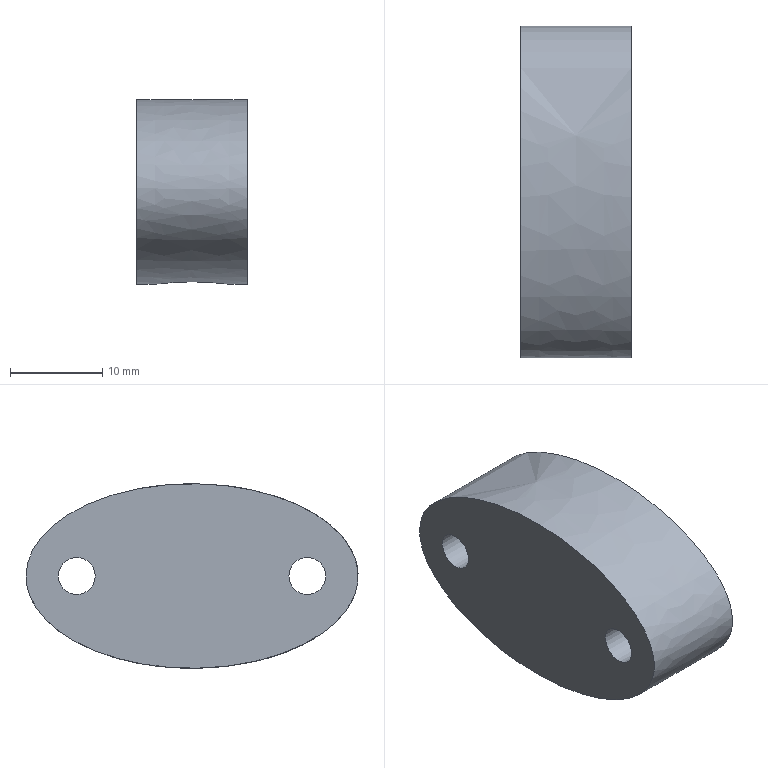Part | STEP file | 1-56.15 | 1 solid | 9 faces | box 12 x 36 x 20 mm | volume 5657 mm3 | cylinder 5 | plane 3 | spline 1 | commonest cylinder face diameters 8 x3 4 x2
STEP:
#1=CARTESIAN_POINT('',(0.,0.,0.));
#2=DIRECTION('',(0.,0.,1.));
#3=DIRECTION('',(1.,0.,0.));
#4=AXIS2_PLACEMENT_3D('',#1,#2,#3);
#5=CARTESIAN_POINT('',(-12.,18.,0.));
#6=VERTEX_POINT('',#5);
#7=CARTESIAN_POINT('',(-12.,0.,0.));
#8=DIRECTION('',(1.,0.,0.));
#9=DIRECTION('',(0.,1.,0.));
#10=AXIS2_PLACEMENT_3D('',#7,#8,#9);
#11=ELLIPSE('',#10,18.,10.);
#12=CARTESIAN_POINT('',(-12.,0.,-8.));
#13=DIRECTION('',(1.,0.,0.));
#14=DIRECTION('',(0.,0.,-1.));
#15=AXIS2_PLACEMENT_3D('',#12,#13,#14);
#16=PLANE('',#15);
#17=CARTESIAN_POINT('',(-8.,0.));
#18=DIRECTION('',(0.,1.));
#19=AXIS2_PLACEMENT_2D('',#17,#18);
#20=ELLIPSE('',#19,18.,10.);
#21=(GEOMETRIC_REPRESENTATION_CONTEXT(2)PARAMETRIC_REPRESENTATION_CONTEXT()REPRESENTATION_CONTEXT('',''));
#22=DEFINITIONAL_REPRESENTATION('',(#20),#21);
#23=PCURVE('',#16,#22);
#24=CARTESIAN_POINT('',(0.,18.,0.));
#25=CARTESIAN_POINT('',(-12.,18.,0.));
#26=CARTESIAN_POINT('',(0.,18.,10.));
#27=CARTESIAN_POINT('',(-12.,18.,10.));
#28=CARTESIAN_POINT('',(0.,0.,10.));
#29=CARTESIAN_POINT('',(-12.,0.,10.));
#30=CARTESIAN_POINT('',(0.,-18.,10.));
#31=CARTESIAN_POINT('',(-12.,-18.,10.));
#32=CARTESIAN_POINT('',(0.,-18.,0.));
#33=CARTESIAN_POINT('',(-12.,-18.,0.));
#34=CARTESIAN_POINT('',(0.,-18.,-10.));
#35=CARTESIAN_POINT('',(-12.,-18.,-10.));
#36=CARTESIAN_POINT('',(0.,0.,-10.));
#37=CARTESIAN_POINT('',(-12.,0.,-10.));
#38=CARTESIAN_POINT('',(0.,18.,-10.));
#39=CARTESIAN_POINT('',(-12.,18.,-10.));
#40=CARTESIAN_POINT('',(0.,18.,0.));
#41=CARTESIAN_POINT('',(-12.,18.,0.));
#42=(BOUNDED_SURFACE()B_SPLINE_SURFACE(2,1,((#24,#25),(#26,#27),(#28,#29),(#30,#31),(#32,#33),(#34,#35),(#36,#37),(#38,#39),(#40,#41)),.UNSPECIFIED.,.T.,.F.,.F.)B_SPLINE_SURFACE_WITH_KNOTS((1,2,2,2,2,2,1),(2,2),(-0.25,0.,0.25,0.5,0.75,1.,1.25),(0.,1.),.UNSPECIFIED.)GEOMETRIC_REPRESENTATION_ITEM()RATIONAL_B_SPLINE_SURFACE(((1.,1.),(0.7071,0.7071),(1.,1.),(0.7071,0.7071),(1.,1.),(0.7071,0.7071),(1.,1.),(0.7071,0.7071),(1.,1.)))REPRESENTATION_ITEM('')SURFACE());
#43=CARTESIAN_POINT('',(0.,1.));
#44=CARTESIAN_POINT('',(0.01678,1.));
#45=CARTESIAN_POINT('',(0.04854,1.));
#46=CARTESIAN_POINT('',(0.09277,1.));
#47=CARTESIAN_POINT('',(0.1357,1.));
#48=CARTESIAN_POINT('',(0.1791,1.));
#49=CARTESIAN_POINT('',(0.2245,1.));
#50=CARTESIAN_POINT('',(0.2755,1.));
#51=CARTESIAN_POINT('',(0.3209,1.));
#52=CARTESIAN_POINT('',(0.3643,1.));
#53=CARTESIAN_POINT('',(0.4073,1.));
#54=CARTESIAN_POINT('',(0.4512,1.));
#55=CARTESIAN_POINT('',(0.5,1.));
#56=CARTESIAN_POINT('',(0.5488,1.));
#57=CARTESIAN_POINT('',(0.5927,1.));
#58=CARTESIAN_POINT('',(0.6357,1.));
#59=CARTESIAN_POINT('',(0.6791,1.));
#60=CARTESIAN_POINT('',(0.7245,1.));
#61=CARTESIAN_POINT('',(0.7755,1.));
#62=CARTESIAN_POINT('',(0.8209,1.));
#63=CARTESIAN_POINT('',(0.8643,1.));
#64=CARTESIAN_POINT('',(0.9072,1.));
#65=CARTESIAN_POINT('',(0.9515,1.));
#66=CARTESIAN_POINT('',(0.9832,1.));
#67=CARTESIAN_POINT('',(1.,1.));
#68=B_SPLINE_CURVE_WITH_KNOTS('',3,(#43,#44,#45,#46,#47,#48,#49,#50,#51,#52,#53,#54,#55,#56,#57,#58,#59,#60,#61,#62,#63,#64,#65,#66,#67),.UNSPECIFIED.,.F.,.F.,(4,1,1,1,1,1,1,1,1,1,1,1,1,1,1,1,1,1,1,1,1,1,4),(0.,0.2856,0.5712,0.8568,1.142,1.428,1.714,1.999,2.285,2.57,2.856,3.142,3.427,3.713,3.998,4.284,4.57,4.855,5.141,5.426,5.712,5.998,6.283),.QUASI_UNIFORM_KNOTS.);
#69=(GEOMETRIC_REPRESENTATION_CONTEXT(2)PARAMETRIC_REPRESENTATION_CONTEXT()REPRESENTATION_CONTEXT('',''));
#70=DEFINITIONAL_REPRESENTATION('',(#68),#69);
#71=PCURVE('',#42,#70);
#72=SURFACE_CURVE('',#11,(#23,#71),.PCURVE_S1.);
#73=EDGE_CURVE('',#6,#6,#72,.T.);
#74=ORIENTED_EDGE('',*,*,#73,.T.);
#75=EDGE_LOOP('',(#74));
#76=FACE_BOUND('',#75,.F.);
#77=CARTESIAN_POINT('',(-12.,14.5,0.));
#78=VERTEX_POINT('',#77);
#79=CARTESIAN_POINT('',(-12.,12.5,0.));
#80=DIRECTION('',(-1.,0.,0.));
#81=DIRECTION('',(0.,1.,0.));
#82=AXIS2_PLACEMENT_3D('',#79,#80,#81);
#83=CIRCLE('',#82,2.);
#84=CARTESIAN_POINT('',(-8.,14.5));
#85=CARTESIAN_POINT('',(-4.536,14.5));
#86=CARTESIAN_POINT('',(-6.268,11.5));
#87=CARTESIAN_POINT('',(-8.,8.5));
#88=CARTESIAN_POINT('',(-9.732,11.5));
#89=CARTESIAN_POINT('',(-11.464,14.5));
#90=CARTESIAN_POINT('',(-8.,14.5));
#91=(BOUNDED_CURVE()B_SPLINE_CURVE(2,(#84,#85,#86,#87,#88,#89,#90),.UNSPECIFIED.,.T.,.F.)B_SPLINE_CURVE_WITH_KNOTS((1,2,2,2,2,1),(-2.094,0.,2.094,4.189,6.283,8.378),.UNSPECIFIED.)CURVE()GEOMETRIC_REPRESENTATION_ITEM()RATIONAL_B_SPLINE_CURVE((1.,0.5,1.,0.5,1.,0.5,1.))REPRESENTATION_ITEM(''));
#92=(GEOMETRIC_REPRESENTATION_CONTEXT(2)PARAMETRIC_REPRESENTATION_CONTEXT()REPRESENTATION_CONTEXT('',''));
#93=DEFINITIONAL_REPRESENTATION('',(#91),#92);
#94=PCURVE('',#16,#93);
#95=CARTESIAN_POINT('',(0.,12.5,0.));
#96=DIRECTION('',(-1.,0.,0.));
#97=DIRECTION('',(0.,1.,0.));
#98=AXIS2_PLACEMENT_3D('',#95,#96,#97);
#99=CYLINDRICAL_SURFACE('',#98,2.);
#100=CARTESIAN_POINT('',(0.,12.));
#101=DIRECTION('',(1.,0.));
#102=VECTOR('',#101,1.);
#103=LINE('',#100,#102);
#104=(GEOMETRIC_REPRESENTATION_CONTEXT(2)PARAMETRIC_REPRESENTATION_CONTEXT()REPRESENTATION_CONTEXT('',''));
#105=DEFINITIONAL_REPRESENTATION('',(#103),#104);
#106=PCURVE('',#99,#105);
#107=SURFACE_CURVE('',#83,(#94,#106),.PCURVE_S1.);
#108=EDGE_CURVE('',#78,#78,#107,.T.);
#109=ORIENTED_EDGE('',*,*,#108,.T.);
#110=EDGE_LOOP('',(#109));
#111=FACE_BOUND('',#110,.F.);
#112=CARTESIAN_POINT('',(-12.,-10.5,0.));
#113=VERTEX_POINT('',#112);
#114=CARTESIAN_POINT('',(-12.,-12.5,0.));
#115=DIRECTION('',(-1.,0.,0.));
#116=DIRECTION('',(0.,1.,0.));
#117=AXIS2_PLACEMENT_3D('',#114,#115,#116);
#118=CIRCLE('',#117,2.);
#119=CARTESIAN_POINT('',(-8.,-10.5));
#120=CARTESIAN_POINT('',(-4.536,-10.5));
#121=CARTESIAN_POINT('',(-6.268,-13.5));
#122=CARTESIAN_POINT('',(-8.,-16.5));
#123=CARTESIAN_POINT('',(-9.732,-13.5));
#124=CARTESIAN_POINT('',(-11.464,-10.5));
#125=CARTESIAN_POINT('',(-8.,-10.5));
#126=(BOUNDED_CURVE()B_SPLINE_CURVE(2,(#119,#120,#121,#122,#123,#124,#125),.UNSPECIFIED.,.T.,.F.)B_SPLINE_CURVE_WITH_KNOTS((1,2,2,2,2,1),(-2.094,0.,2.094,4.189,6.283,8.378),.UNSPECIFIED.)CURVE()GEOMETRIC_REPRESENTATION_ITEM()RATIONAL_B_SPLINE_CURVE((1.,0.5,1.,0.5,1.,0.5,1.))REPRESENTATION_ITEM(''));
#127=(GEOMETRIC_REPRESENTATION_CONTEXT(2)PARAMETRIC_REPRESENTATION_CONTEXT()REPRESENTATION_CONTEXT('',''));
#128=DEFINITIONAL_REPRESENTATION('',(#126),#127);
#129=PCURVE('',#16,#128);
#130=CARTESIAN_POINT('',(0.,-12.5,0.));
#131=DIRECTION('',(-1.,0.,0.));
#132=DIRECTION('',(0.,1.,0.));
#133=AXIS2_PLACEMENT_3D('',#130,#131,#132);
#134=CYLINDRICAL_SURFACE('',#133,2.);
#135=CARTESIAN_POINT('',(0.,12.));
#136=DIRECTION('',(1.,0.));
#137=VECTOR('',#136,1.);
#138=LINE('',#135,#137);
#139=(GEOMETRIC_REPRESENTATION_CONTEXT(2)PARAMETRIC_REPRESENTATION_CONTEXT()REPRESENTATION_CONTEXT('',''));
#140=DEFINITIONAL_REPRESENTATION('',(#138),#139);
#141=PCURVE('',#134,#140);
#142=SURFACE_CURVE('',#118,(#129,#141),.PCURVE_S1.);
#143=EDGE_CURVE('',#113,#113,#142,.T.);
#144=ORIENTED_EDGE('',*,*,#143,.T.);
#145=EDGE_LOOP('',(#144));
#146=FACE_BOUND('',#145,.F.);
#147=ADVANCED_FACE('',(#76,#111,#146),#16,.F.);
#148=CARTESIAN_POINT('',(0.,-10.5,0.));
#149=VERTEX_POINT('',#148);
#150=CARTESIAN_POINT('',(0.,-12.5,0.));
#151=DIRECTION('',(-1.,0.,0.));
#152=DIRECTION('',(0.,1.,0.));
#153=AXIS2_PLACEMENT_3D('',#150,#151,#152);
#154=CIRCLE('',#153,2.);
#155=CARTESIAN_POINT('',(0.,0.));
#156=DIRECTION('',(1.,0.));
#157=VECTOR('',#156,1.);
#158=LINE('',#155,#157);
#159=(GEOMETRIC_REPRESENTATION_CONTEXT(2)PARAMETRIC_REPRESENTATION_CONTEXT()REPRESENTATION_CONTEXT('',''));
#160=DEFINITIONAL_REPRESENTATION('',(#158),#159);
#161=PCURVE('',#134,#160);
#162=CARTESIAN_POINT('',(0.,0.,-8.));
#163=DIRECTION('',(1.,0.,0.));
#164=DIRECTION('',(0.,0.,-1.));
#165=AXIS2_PLACEMENT_3D('',#162,#163,#164);
#166=PLANE('',#165);
#167=CARTESIAN_POINT('',(-8.,-10.5));
#168=CARTESIAN_POINT('',(-4.536,-10.5));
#169=CARTESIAN_POINT('',(-6.268,-13.5));
#170=CARTESIAN_POINT('',(-8.,-16.5));
#171=CARTESIAN_POINT('',(-9.732,-13.5));
#172=CARTESIAN_POINT('',(-11.464,-10.5));
#173=CARTESIAN_POINT('',(-8.,-10.5));
#174=(BOUNDED_CURVE()B_SPLINE_CURVE(2,(#167,#168,#169,#170,#171,#172,#173),.UNSPECIFIED.,.T.,.F.)B_SPLINE_CURVE_WITH_KNOTS((1,2,2,2,2,1),(-2.094,0.,2.094,4.189,6.283,8.378),.UNSPECIFIED.)CURVE()GEOMETRIC_REPRESENTATION_ITEM()RATIONAL_B_SPLINE_CURVE((1.,0.5,1.,0.5,1.,0.5,1.))REPRESENTATION_ITEM(''));
#175=(GEOMETRIC_REPRESENTATION_CONTEXT(2)PARAMETRIC_REPRESENTATION_CONTEXT()REPRESENTATION_CONTEXT('',''));
#176=DEFINITIONAL_REPRESENTATION('',(#174),#175);
#177=PCURVE('',#166,#176);
#178=SURFACE_CURVE('',#154,(#161,#177),.PCURVE_S1.);
#179=EDGE_CURVE('',#149,#149,#178,.T.);
#180=ORIENTED_EDGE('',*,*,#179,.T.);
#181=CARTESIAN_POINT('',(0.,-10.5,0.));
#182=DIRECTION('',(-1.,0.,0.));
#183=VECTOR('',#182,1.);
#184=LINE('',#181,#183);
#185=CARTESIAN_POINT('',(6.283,0.));
#186=DIRECTION('',(0.,1.));
#187=VECTOR('',#186,1.);
#188=LINE('',#185,#187);
#189=(GEOMETRIC_REPRESENTATION_CONTEXT(2)PARAMETRIC_REPRESENTATION_CONTEXT()REPRESENTATION_CONTEXT('',''));
#190=DEFINITIONAL_REPRESENTATION('',(#188),#189);
#191=PCURVE('',#134,#190);
#192=CARTESIAN_POINT('',(0.,0.));
#193=DIRECTION('',(0.,1.));
#194=VECTOR('',#193,1.);
#195=LINE('',#192,#194);
#196=(GEOMETRIC_REPRESENTATION_CONTEXT(2)PARAMETRIC_REPRESENTATION_CONTEXT()REPRESENTATION_CONTEXT('',''));
#197=DEFINITIONAL_REPRESENTATION('',(#195),#196);
#198=PCURVE('',#134,#197);
#199=SEAM_CURVE('',#184,(#191,#198),.PCURVE_S1.);
#200=EDGE_CURVE('',#149,#113,#199,.T.);
#201=ORIENTED_EDGE('',*,*,#200,.T.);
#202=ORIENTED_EDGE('',*,*,#143,.F.);
#203=ORIENTED_EDGE('',*,*,#200,.F.);
#204=EDGE_LOOP('',(#180,#201,#202,#203));
#205=FACE_BOUND('',#204,.F.);
#206=ADVANCED_FACE('',(#205),#134,.F.);
#207=CARTESIAN_POINT('',(0.,18.,0.));
#208=VERTEX_POINT('',#207);
#209=CARTESIAN_POINT('',(0.,0.,0.));
#210=DIRECTION('',(1.,0.,0.));
#211=DIRECTION('',(0.,1.,0.));
#212=AXIS2_PLACEMENT_3D('',#209,#210,#211);
#213=ELLIPSE('',#212,18.,10.);
#214=CARTESIAN_POINT('',(-8.,0.));
#215=DIRECTION('',(0.,1.));
#216=AXIS2_PLACEMENT_2D('',#214,#215);
#217=ELLIPSE('',#216,18.,10.);
#218=(GEOMETRIC_REPRESENTATION_CONTEXT(2)PARAMETRIC_REPRESENTATION_CONTEXT()REPRESENTATION_CONTEXT('',''));
#219=DEFINITIONAL_REPRESENTATION('',(#217),#218);
#220=PCURVE('',#166,#219);
#221=CARTESIAN_POINT('',(0.,0.));
#222=CARTESIAN_POINT('',(0.01678,0.));
#223=CARTESIAN_POINT('',(0.04854,0.));
#224=CARTESIAN_POINT('',(0.09277,0.));
#225=CARTESIAN_POINT('',(0.1357,0.));
#226=CARTESIAN_POINT('',(0.1791,0.));
#227=CARTESIAN_POINT('',(0.2245,0.));
#228=CARTESIAN_POINT('',(0.2755,0.));
#229=CARTESIAN_POINT('',(0.3209,0.));
#230=CARTESIAN_POINT('',(0.3643,0.));
#231=CARTESIAN_POINT('',(0.4073,0.));
#232=CARTESIAN_POINT('',(0.4512,0.));
#233=CARTESIAN_POINT('',(0.5,0.));
#234=CARTESIAN_POINT('',(0.5488,0.));
#235=CARTESIAN_POINT('',(0.5927,0.));
#236=CARTESIAN_POINT('',(0.6357,0.));
#237=CARTESIAN_POINT('',(0.6791,0.));
#238=CARTESIAN_POINT('',(0.7245,0.));
#239=CARTESIAN_POINT('',(0.7755,0.));
#240=CARTESIAN_POINT('',(0.8209,0.));
#241=CARTESIAN_POINT('',(0.8643,0.));
#242=CARTESIAN_POINT('',(0.9072,0.));
#243=CARTESIAN_POINT('',(0.9515,0.));
#244=CARTESIAN_POINT('',(0.9832,0.));
#245=CARTESIAN_POINT('',(1.,0.));
#246=B_SPLINE_CURVE_WITH_KNOTS('',3,(#221,#222,#223,#224,#225,#226,#227,#228,#229,#230,#231,#232,#233,#234,#235,#236,#237,#238,#239,#240,#241,#242,#243,#244,#245),.UNSPECIFIED.,.F.,.F.,(4,1,1,1,1,1,1,1,1,1,1,1,1,1,1,1,1,1,1,1,1,1,4),(0.,0.2856,0.5712,0.8568,1.142,1.428,1.714,1.999,2.285,2.57,2.856,3.142,3.427,3.713,3.998,4.284,4.57,4.855,5.141,5.426,5.712,5.998,6.283),.QUASI_UNIFORM_KNOTS.);
#247=(GEOMETRIC_REPRESENTATION_CONTEXT(2)PARAMETRIC_REPRESENTATION_CONTEXT()REPRESENTATION_CONTEXT('',''));
#248=DEFINITIONAL_REPRESENTATION('',(#246),#247);
#249=PCURVE('',#42,#248);
#250=SURFACE_CURVE('',#213,(#220,#249),.PCURVE_S1.);
#251=EDGE_CURVE('',#208,#208,#250,.T.);
#252=ORIENTED_EDGE('',*,*,#251,.T.);
#253=EDGE_LOOP('',(#252));
#254=FACE_BOUND('',#253,.T.);
#255=CARTESIAN_POINT('',(0.,4.,0.));
#256=VERTEX_POINT('',#255);
#257=CARTESIAN_POINT('',(0.,0.,0.));
#258=DIRECTION('',(1.,0.,0.));
#259=DIRECTION('',(0.,1.,0.));
#260=AXIS2_PLACEMENT_3D('',#257,#258,#259);
#261=CIRCLE('',#260,4.);
#262=CARTESIAN_POINT('',(-8.,0.));
#263=DIRECTION('',(0.,1.));
#264=AXIS2_PLACEMENT_2D('',#262,#263);
#265=CIRCLE('',#264,4.);
#266=(GEOMETRIC_REPRESENTATION_CONTEXT(2)PARAMETRIC_REPRESENTATION_CONTEXT()REPRESENTATION_CONTEXT('',''));
#267=DEFINITIONAL_REPRESENTATION('',(#265),#266);
#268=PCURVE('',#166,#267);
#269=CARTESIAN_POINT('',(0.,0.,0.));
#270=DIRECTION('',(-1.,0.,0.));
#271=DIRECTION('',(0.,1.,0.));
#272=AXIS2_PLACEMENT_3D('',#269,#270,#271);
#273=CYLINDRICAL_SURFACE('',#272,4.);
#274=CARTESIAN_POINT('',(6.283,0.));
#275=DIRECTION('',(-1.,0.));
#276=VECTOR('',#275,1.);
#277=LINE('',#274,#276);
#278=(GEOMETRIC_REPRESENTATION_CONTEXT(2)PARAMETRIC_REPRESENTATION_CONTEXT()REPRESENTATION_CONTEXT('',''));
#279=DEFINITIONAL_REPRESENTATION('',(#277),#278);
#280=PCURVE('',#273,#279);
#281=SURFACE_CURVE('',#261,(#268,#280),.PCURVE_S1.);
#282=EDGE_CURVE('',#256,#256,#281,.T.);
#283=ORIENTED_EDGE('',*,*,#282,.F.);
#284=EDGE_LOOP('',(#283));
#285=FACE_BOUND('',#284,.T.);
#286=CARTESIAN_POINT('',(0.,14.5,0.));
#287=VERTEX_POINT('',#286);
#288=CARTESIAN_POINT('',(0.,12.5,0.));
#289=DIRECTION('',(-1.,0.,0.));
#290=DIRECTION('',(0.,1.,0.));
#291=AXIS2_PLACEMENT_3D('',#288,#289,#290);
#292=CIRCLE('',#291,2.);
#293=CARTESIAN_POINT('',(-8.,14.5));
#294=CARTESIAN_POINT('',(-4.536,14.5));
#295=CARTESIAN_POINT('',(-6.268,11.5));
#296=CARTESIAN_POINT('',(-8.,8.5));
#297=CARTESIAN_POINT('',(-9.732,11.5));
#298=CARTESIAN_POINT('',(-11.464,14.5));
#299=CARTESIAN_POINT('',(-8.,14.5));
#300=(BOUNDED_CURVE()B_SPLINE_CURVE(2,(#293,#294,#295,#296,#297,#298,#299),.UNSPECIFIED.,.T.,.F.)B_SPLINE_CURVE_WITH_KNOTS((1,2,2,2,2,1),(-2.094,0.,2.094,4.189,6.283,8.378),.UNSPECIFIED.)CURVE()GEOMETRIC_REPRESENTATION_ITEM()RATIONAL_B_SPLINE_CURVE((1.,0.5,1.,0.5,1.,0.5,1.))REPRESENTATION_ITEM(''));
#301=(GEOMETRIC_REPRESENTATION_CONTEXT(2)PARAMETRIC_REPRESENTATION_CONTEXT()REPRESENTATION_CONTEXT('',''));
#302=DEFINITIONAL_REPRESENTATION('',(#300),#301);
#303=PCURVE('',#166,#302);
#304=CARTESIAN_POINT('',(0.,0.));
#305=DIRECTION('',(1.,0.));
#306=VECTOR('',#305,1.);
#307=LINE('',#304,#306);
#308=(GEOMETRIC_REPRESENTATION_CONTEXT(2)PARAMETRIC_REPRESENTATION_CONTEXT()REPRESENTATION_CONTEXT('',''));
#309=DEFINITIONAL_REPRESENTATION('',(#307),#308);
#310=PCURVE('',#99,#309);
#311=SURFACE_CURVE('',#292,(#303,#310),.PCURVE_S1.);
#312=EDGE_CURVE('',#287,#287,#311,.T.);
#313=ORIENTED_EDGE('',*,*,#312,.T.);
#314=EDGE_LOOP('',(#313));
#315=FACE_BOUND('',#314,.T.);
#316=ORIENTED_EDGE('',*,*,#179,.T.);
#317=EDGE_LOOP('',(#316));
#318=FACE_BOUND('',#317,.T.);
#319=ADVANCED_FACE('',(#254,#285,#315,#318),#166,.T.);
#320=CARTESIAN_POINT('',(-6.,4.,0.));
#321=VERTEX_POINT('',#320);
#322=CARTESIAN_POINT('',(0.,4.,0.));
#323=DIRECTION('',(-1.,0.,0.));
#324=VECTOR('',#323,1.);
#325=LINE('',#322,#324);
#326=CARTESIAN_POINT('',(6.283,0.));
#327=DIRECTION('',(0.,1.));
#328=VECTOR('',#327,1.);
#329=LINE('',#326,#328);
#330=(GEOMETRIC_REPRESENTATION_CONTEXT(2)PARAMETRIC_REPRESENTATION_CONTEXT()REPRESENTATION_CONTEXT('',''));
#331=DEFINITIONAL_REPRESENTATION('',(#329),#330);
#332=PCURVE('',#273,#331);
#333=CARTESIAN_POINT('',(0.,0.));
#334=DIRECTION('',(0.,1.));
#335=VECTOR('',#334,1.);
#336=LINE('',#333,#335);
#337=(GEOMETRIC_REPRESENTATION_CONTEXT(2)PARAMETRIC_REPRESENTATION_CONTEXT()REPRESENTATION_CONTEXT('',''));
#338=DEFINITIONAL_REPRESENTATION('',(#336),#337);
#339=PCURVE('',#273,#338);
#340=SEAM_CURVE('',#325,(#332,#339),.PCURVE_S1.);
#341=EDGE_CURVE('',#256,#321,#340,.T.);
#342=ORIENTED_EDGE('',*,*,#341,.T.);
#343=CARTESIAN_POINT('',(-10.,4.,0.));
#344=VERTEX_POINT('',#343);
#345=CARTESIAN_POINT('',(-6.,4.,0.));
#346=DIRECTION('',(-1.,0.,0.));
#347=VECTOR('',#346,1.);
#348=LINE('',#345,#347);
#349=CARTESIAN_POINT('',(6.283,6.));
#350=DIRECTION('',(0.,1.));
#351=VECTOR('',#350,1.);
#352=LINE('',#349,#351);
#353=(GEOMETRIC_REPRESENTATION_CONTEXT(2)PARAMETRIC_REPRESENTATION_CONTEXT()REPRESENTATION_CONTEXT('',''));
#354=DEFINITIONAL_REPRESENTATION('',(#352),#353);
#355=PCURVE('',#273,#354);
#356=CARTESIAN_POINT('',(0.,0.,0.));
#357=DIRECTION('',(-1.,0.,0.));
#358=DIRECTION('',(0.,1.,0.));
#359=AXIS2_PLACEMENT_3D('',#356,#357,#358);
#360=CYLINDRICAL_SURFACE('',#359,4.);
#361=CARTESIAN_POINT('',(0.,6.));
#362=DIRECTION('',(0.,1.));
#363=VECTOR('',#362,1.);
#364=LINE('',#361,#363);
#365=(GEOMETRIC_REPRESENTATION_CONTEXT(2)PARAMETRIC_REPRESENTATION_CONTEXT()REPRESENTATION_CONTEXT('',''));
#366=DEFINITIONAL_REPRESENTATION('',(#364),#365);
#367=PCURVE('',#360,#366);
#368=SURFACE_CURVE('',#348,(#355,#367),.PCURVE_S1.);
#369=EDGE_CURVE('',#321,#344,#368,.T.);
#370=ORIENTED_EDGE('',*,*,#369,.T.);
#371=CARTESIAN_POINT('',(-10.,0.00000086,-4.));
#372=VERTEX_POINT('',#371);
#373=CARTESIAN_POINT('',(-10.,0.,0.));
#374=DIRECTION('',(1.,0.,0.));
#375=DIRECTION('',(0.,1.,0.));
#376=AXIS2_PLACEMENT_3D('',#373,#374,#375);
#377=CIRCLE('',#376,4.);
#378=CARTESIAN_POINT('',(6.283,10.));
#379=DIRECTION('',(-1.,0.));
#380=VECTOR('',#379,1.);
#381=LINE('',#378,#380);
#382=(GEOMETRIC_REPRESENTATION_CONTEXT(2)PARAMETRIC_REPRESENTATION_CONTEXT()REPRESENTATION_CONTEXT('',''));
#383=DEFINITIONAL_REPRESENTATION('',(#381),#382);
#384=PCURVE('',#273,#383);
#385=CARTESIAN_POINT('',(-10.,-1.072,0.));
#386=DIRECTION('',(1.,0.,0.));
#387=DIRECTION('',(0.,0.,-1.));
#388=AXIS2_PLACEMENT_3D('',#385,#386,#387);
#389=PLANE('',#388);
#390=CARTESIAN_POINT('',(0.,1.072));
#391=DIRECTION('',(0.,1.));
#392=AXIS2_PLACEMENT_2D('',#390,#391);
#393=CIRCLE('',#392,4.);
#394=(GEOMETRIC_REPRESENTATION_CONTEXT(2)PARAMETRIC_REPRESENTATION_CONTEXT()REPRESENTATION_CONTEXT('',''));
#395=DEFINITIONAL_REPRESENTATION('',(#393),#394);
#396=PCURVE('',#389,#395);
#397=SURFACE_CURVE('',#377,(#384,#396),.PCURVE_S1.);
#398=EDGE_CURVE('',#344,#372,#397,.T.);
#399=ORIENTED_EDGE('',*,*,#398,.T.);
#400=CARTESIAN_POINT('',(-6.,-4.,0.));
#401=VERTEX_POINT('',#400);
#402=CARTESIAN_POINT('',(-10.001,0.000001721,-4.001));
#403=CARTESIAN_POINT('',(-10.001,-0.5849,-4.001));
#404=CARTESIAN_POINT('',(-9.873,-1.182,-3.873));
#405=CARTESIAN_POINT('',(-8.829,-3.329,-2.829));
#406=CARTESIAN_POINT('',(-7.292,-4.,-1.292));
#407=CARTESIAN_POINT('',(-6.,-4.,0.));
#408=B_SPLINE_CURVE_WITH_KNOTS('',3,(#402,#403,#404,#405,#406,#407),.UNSPECIFIED.,.F.,.F.,(4,2,4),(1.382,1.741,2.741),.UNSPECIFIED.);
#409=CARTESIAN_POINT('',(1.571,10.001));
#410=CARTESIAN_POINT('',(1.596,10.001));
#411=CARTESIAN_POINT('',(1.646,9.993));
#412=CARTESIAN_POINT('',(1.723,9.959));
#413=CARTESIAN_POINT('',(1.8,9.9));
#414=CARTESIAN_POINT('',(1.878,9.817));
#415=CARTESIAN_POINT('',(1.957,9.709));
#416=CARTESIAN_POINT('',(2.039,9.574));
#417=CARTESIAN_POINT('',(2.118,9.419));
#418=CARTESIAN_POINT('',(2.195,9.249));
#419=CARTESIAN_POINT('',(2.271,9.065));
#420=CARTESIAN_POINT('',(2.344,8.867));
#421=CARTESIAN_POINT('',(2.416,8.658));
#422=CARTESIAN_POINT('',(2.487,8.438));
#423=CARTESIAN_POINT('',(2.557,8.21));
#424=CARTESIAN_POINT('',(2.626,7.974));
#425=CARTESIAN_POINT('',(2.694,7.733));
#426=CARTESIAN_POINT('',(2.761,7.487));
#427=CARTESIAN_POINT('',(2.827,7.238));
#428=CARTESIAN_POINT('',(2.892,6.988));
#429=CARTESIAN_POINT('',(2.956,6.737));
#430=CARTESIAN_POINT('',(3.019,6.488));
#431=CARTESIAN_POINT('',(3.081,6.241));
#432=CARTESIAN_POINT('',(3.122,6.08));
#433=CARTESIAN_POINT('',(3.142,6.));
#434=B_SPLINE_CURVE_WITH_KNOTS('',3,(#409,#410,#411,#412,#413,#414,#415,#416,#417,#418,#419,#420,#421,#422,#423,#424,#425,#426,#427,#428,#429,#430,#431,#432,#433),.UNSPECIFIED.,.F.,.F.,(4,1,1,1,1,1,1,1,1,1,1,1,1,1,1,1,1,1,1,1,1,1,4),(1.382,1.444,1.505,1.567,1.629,1.691,1.753,1.814,1.876,1.938,2.,2.062,2.123,2.185,2.247,2.309,2.371,2.432,2.494,2.556,2.618,2.68,2.741),.QUASI_UNIFORM_KNOTS.);
#435=(GEOMETRIC_REPRESENTATION_CONTEXT(2)PARAMETRIC_REPRESENTATION_CONTEXT()REPRESENTATION_CONTEXT('',''));
#436=DEFINITIONAL_REPRESENTATION('',(#434),#435);
#437=PCURVE('',#273,#436);
#438=CARTESIAN_POINT('',(-6.,0.,0.));
#439=DIRECTION('',(0.,0.,-1.));
#440=DIRECTION('',(0.,1.,0.));
#441=AXIS2_PLACEMENT_3D('',#438,#439,#440);
#442=CYLINDRICAL_SURFACE('',#441,4.);
#443=CARTESIAN_POINT('',(4.712,4.001));
#444=CARTESIAN_POINT('',(4.687,4.001));
#445=CARTESIAN_POINT('',(4.637,3.993));
#446=CARTESIAN_POINT('',(4.561,3.959));
#447=CARTESIAN_POINT('',(4.483,3.9));
#448=CARTESIAN_POINT('',(4.405,3.817));
#449=CARTESIAN_POINT('',(4.326,3.709));
#450=CARTESIAN_POINT('',(4.245,3.574));
#451=CARTESIAN_POINT('',(4.165,3.419));
#452=CARTESIAN_POINT('',(4.088,3.249));
#453=CARTESIAN_POINT('',(4.012,3.065));
#454=CARTESIAN_POINT('',(3.939,2.867));
#455=CARTESIAN_POINT('',(3.867,2.658));
#456=CARTESIAN_POINT('',(3.796,2.438));
#457=CARTESIAN_POINT('',(3.726,2.21));
#458=CARTESIAN_POINT('',(3.657,1.974));
#459=CARTESIAN_POINT('',(3.589,1.733));
#460=CARTESIAN_POINT('',(3.522,1.487));
#461=CARTESIAN_POINT('',(3.456,1.238));
#462=CARTESIAN_POINT('',(3.391,0.9877));
#463=CARTESIAN_POINT('',(3.327,0.7372));
#464=CARTESIAN_POINT('',(3.264,0.4879));
#465=CARTESIAN_POINT('',(3.202,0.2414));
#466=CARTESIAN_POINT('',(3.162,0.07984));
#467=CARTESIAN_POINT('',(3.142,0.));
#468=B_SPLINE_CURVE_WITH_KNOTS('',3,(#443,#444,#445,#446,#447,#448,#449,#450,#451,#452,#453,#454,#455,#456,#457,#458,#459,#460,#461,#462,#463,#464,#465,#466,#467),.UNSPECIFIED.,.F.,.F.,(4,1,1,1,1,1,1,1,1,1,1,1,1,1,1,1,1,1,1,1,1,1,4),(1.382,1.444,1.505,1.567,1.629,1.691,1.753,1.814,1.876,1.938,2.,2.062,2.123,2.185,2.247,2.309,2.371,2.432,2.494,2.556,2.618,2.68,2.741),.QUASI_UNIFORM_KNOTS.);
#469=(GEOMETRIC_REPRESENTATION_CONTEXT(2)PARAMETRIC_REPRESENTATION_CONTEXT()REPRESENTATION_CONTEXT('',''));
#470=DEFINITIONAL_REPRESENTATION('',(#468),#469);
#471=PCURVE('',#442,#470);
#472=SURFACE_CURVE('',#408,(#437,#471),.PCURVE_S1.);
#473=EDGE_CURVE('',#372,#401,#472,.T.);
#474=ORIENTED_EDGE('',*,*,#473,.T.);
#475=CARTESIAN_POINT('',(-6.,-4.,0.));
#476=CARTESIAN_POINT('',(-5.056,-4.,-0.9444));
#477=CARTESIAN_POINT('',(-4.054,-3.66,-1.946));
#478=CARTESIAN_POINT('',(-1.944,-1.677,-4.056));
#479=CARTESIAN_POINT('',(-1.545,0.4188,-4.455));
#480=CARTESIAN_POINT('',(-3.428,3.432,-2.572));
#481=CARTESIAN_POINT('',(-4.799,4.,-1.201));
#482=CARTESIAN_POINT('',(-6.,4.,0.));
#483=B_SPLINE_CURVE_WITH_KNOTS('',3,(#475,#476,#477,#478,#479,#480,#481,#482),.UNSPECIFIED.,.F.,.F.,(4,2,2,4),(0.,0.7815,2.078,3.078),.UNSPECIFIED.);
#484=CARTESIAN_POINT('',(3.142,6.));
#485=CARTESIAN_POINT('',(3.099,5.831));
#486=CARTESIAN_POINT('',(3.014,5.489));
#487=CARTESIAN_POINT('',(2.883,4.975));
#488=CARTESIAN_POINT('',(2.75,4.467));
#489=CARTESIAN_POINT('',(2.613,3.976));
#490=CARTESIAN_POINT('',(2.473,3.512));
#491=CARTESIAN_POINT('',(2.327,3.079));
#492=CARTESIAN_POINT('',(2.181,2.712));
#493=CARTESIAN_POINT('',(2.037,2.416));
#494=CARTESIAN_POINT('',(1.892,2.193));
#495=CARTESIAN_POINT('',(1.746,2.049));
#496=CARTESIAN_POINT('',(1.6,1.987));
#497=CARTESIAN_POINT('',(1.453,2.011));
#498=CARTESIAN_POINT('',(1.303,2.126));
#499=CARTESIAN_POINT('',(1.149,2.334));
#500=CARTESIAN_POINT('',(0.9875,2.647));
#501=CARTESIAN_POINT('',(0.8303,3.035));
#502=CARTESIAN_POINT('',(0.6814,3.47));
#503=CARTESIAN_POINT('',(0.5372,3.946));
#504=CARTESIAN_POINT('',(0.397,4.449));
#505=CARTESIAN_POINT('',(0.2605,4.967));
#506=CARTESIAN_POINT('',(0.1276,5.489));
#507=CARTESIAN_POINT('',(0.04201,5.832));
#508=CARTESIAN_POINT('',(0.,6.));
#509=B_SPLINE_CURVE_WITH_KNOTS('',3,(#484,#485,#486,#487,#488,#489,#490,#491,#492,#493,#494,#495,#496,#497,#498,#499,#500,#501,#502,#503,#504,#505,#506,#507,#508),.UNSPECIFIED.,.F.,.F.,(4,1,1,1,1,1,1,1,1,1,1,1,1,1,1,1,1,1,1,1,1,1,4),(0.,0.1399,0.2798,0.4197,0.5596,0.6994,0.8393,0.9792,1.119,1.259,1.399,1.539,1.679,1.819,1.958,2.098,2.238,2.378,2.518,2.658,2.798,2.938,3.078),.QUASI_UNIFORM_KNOTS.);
#510=(GEOMETRIC_REPRESENTATION_CONTEXT(2)PARAMETRIC_REPRESENTATION_CONTEXT()REPRESENTATION_CONTEXT('',''));
#511=DEFINITIONAL_REPRESENTATION('',(#509),#510);
#512=PCURVE('',#273,#511);
#513=CARTESIAN_POINT('',(3.142,0.));
#514=CARTESIAN_POINT('',(3.099,0.169));
#515=CARTESIAN_POINT('',(3.014,0.5108));
#516=CARTESIAN_POINT('',(2.883,1.025));
#517=CARTESIAN_POINT('',(2.75,1.533));
#518=CARTESIAN_POINT('',(2.613,2.024));
#519=CARTESIAN_POINT('',(2.473,2.488));
#520=CARTESIAN_POINT('',(2.327,2.921));
#521=CARTESIAN_POINT('',(2.181,3.288));
#522=CARTESIAN_POINT('',(2.037,3.584));
#523=CARTESIAN_POINT('',(1.892,3.807));
#524=CARTESIAN_POINT('',(1.746,3.951));
#525=CARTESIAN_POINT('',(1.6,4.013));
#526=CARTESIAN_POINT('',(1.453,3.989));
#527=CARTESIAN_POINT('',(1.303,3.874));
#528=CARTESIAN_POINT('',(1.149,3.666));
#529=CARTESIAN_POINT('',(0.9875,3.353));
#530=CARTESIAN_POINT('',(0.8303,2.965));
#531=CARTESIAN_POINT('',(0.6814,2.53));
#532=CARTESIAN_POINT('',(0.5372,2.054));
#533=CARTESIAN_POINT('',(0.397,1.551));
#534=CARTESIAN_POINT('',(0.2605,1.033));
#535=CARTESIAN_POINT('',(0.1276,0.5106));
#536=CARTESIAN_POINT('',(0.04201,0.168));
#537=CARTESIAN_POINT('',(0.,0.));
#538=B_SPLINE_CURVE_WITH_KNOTS('',3,(#513,#514,#515,#516,#517,#518,#519,#520,#521,#522,#523,#524,#525,#526,#527,#528,#529,#530,#531,#532,#533,#534,#535,#536,#537),.UNSPECIFIED.,.F.,.F.,(4,1,1,1,1,1,1,1,1,1,1,1,1,1,1,1,1,1,1,1,1,1,4),(0.,0.1399,0.2798,0.4197,0.5596,0.6994,0.8393,0.9792,1.119,1.259,1.399,1.539,1.679,1.819,1.958,2.098,2.238,2.378,2.518,2.658,2.798,2.938,3.078),.QUASI_UNIFORM_KNOTS.);
#539=(GEOMETRIC_REPRESENTATION_CONTEXT(2)PARAMETRIC_REPRESENTATION_CONTEXT()REPRESENTATION_CONTEXT('',''));
#540=DEFINITIONAL_REPRESENTATION('',(#538),#539);
#541=PCURVE('',#442,#540);
#542=SURFACE_CURVE('',#483,(#512,#541),.PCURVE_S1.);
#543=EDGE_CURVE('',#401,#321,#542,.T.);
#544=ORIENTED_EDGE('',*,*,#543,.T.);
#545=ORIENTED_EDGE('',*,*,#341,.F.);
#546=ORIENTED_EDGE('',*,*,#282,.F.);
#547=EDGE_LOOP('',(#342,#370,#399,#474,#544,#545,#546));
#548=FACE_BOUND('',#547,.F.);
#549=ADVANCED_FACE('',(#548),#273,.F.);
#550=ORIENTED_EDGE('',*,*,#543,.F.);
#551=ORIENTED_EDGE('',*,*,#473,.F.);
#552=CARTESIAN_POINT('',(-6.,4.,0.));
#553=CARTESIAN_POINT('',(-7.044,4.,-1.044));
#554=CARTESIAN_POINT('',(-8.174,3.582,-2.174));
#555=CARTESIAN_POINT('',(-9.636,1.925,-3.636));
#556=CARTESIAN_POINT('',(-9.999,0.9788,-3.999));
#557=CARTESIAN_POINT('',(-10.001,0.000001721,-4.001));
#558=B_SPLINE_CURVE_WITH_KNOTS('',3,(#552,#553,#554,#555,#556,#557),.UNSPECIFIED.,.F.,.F.,(4,2,4),(0.,0.7803,1.382),.UNSPECIFIED.);
#559=CARTESIAN_POINT('',(6.283,0.));
#560=CARTESIAN_POINT('',(6.262,0.08405));
#561=CARTESIAN_POINT('',(6.22,0.2533));
#562=CARTESIAN_POINT('',(6.156,0.5092));
#563=CARTESIAN_POINT('',(6.091,0.7661));
#564=CARTESIAN_POINT('',(6.025,1.023));
#565=CARTESIAN_POINT('',(5.958,1.278));
#566=CARTESIAN_POINT('',(5.891,1.53));
#567=CARTESIAN_POINT('',(5.823,1.778));
#568=CARTESIAN_POINT('',(5.754,2.021));
#569=CARTESIAN_POINT('',(5.684,2.258));
#570=CARTESIAN_POINT('',(5.613,2.486));
#571=CARTESIAN_POINT('',(5.541,2.706));
#572=CARTESIAN_POINT('',(5.467,2.916));
#573=CARTESIAN_POINT('',(5.392,3.115));
#574=CARTESIAN_POINT('',(5.317,3.295));
#575=CARTESIAN_POINT('',(5.241,3.456));
#576=CARTESIAN_POINT('',(5.166,3.597));
#577=CARTESIAN_POINT('',(5.091,3.719));
#578=CARTESIAN_POINT('',(5.016,3.819));
#579=CARTESIAN_POINT('',(4.941,3.899));
#580=CARTESIAN_POINT('',(4.865,3.957));
#581=CARTESIAN_POINT('',(4.789,3.992));
#582=CARTESIAN_POINT('',(4.738,4.));
#583=CARTESIAN_POINT('',(4.712,4.001));
#584=B_SPLINE_CURVE_WITH_KNOTS('',3,(#559,#560,#561,#562,#563,#564,#565,#566,#567,#568,#569,#570,#571,#572,#573,#574,#575,#576,#577,#578,#579,#580,#581,#582,#583),.UNSPECIFIED.,.F.,.F.,(4,1,1,1,1,1,1,1,1,1,1,1,1,1,1,1,1,1,1,1,1,1,4),(0.,0.06281,0.1256,0.1884,0.2512,0.3141,0.3769,0.4397,0.5025,0.5653,0.6281,0.6909,0.7537,0.8165,0.8794,0.9422,1.005,1.068,1.131,1.193,1.256,1.319,1.382),.QUASI_UNIFORM_KNOTS.);
#585=(GEOMETRIC_REPRESENTATION_CONTEXT(2)PARAMETRIC_REPRESENTATION_CONTEXT()REPRESENTATION_CONTEXT('',''));
#586=DEFINITIONAL_REPRESENTATION('',(#584),#585);
#587=PCURVE('',#442,#586);
#588=CARTESIAN_POINT('',(0.,6.));
#589=CARTESIAN_POINT('',(0.02101,6.084));
#590=CARTESIAN_POINT('',(0.06332,6.253));
#591=CARTESIAN_POINT('',(0.1276,6.509));
#592=CARTESIAN_POINT('',(0.1926,6.766));
#593=CARTESIAN_POINT('',(0.2584,7.023));
#594=CARTESIAN_POINT('',(0.3249,7.278));
#595=CARTESIAN_POINT('',(0.3921,7.53));
#596=CARTESIAN_POINT('',(0.4602,7.778));
#597=CARTESIAN_POINT('',(0.5291,8.021));
#598=CARTESIAN_POINT('',(0.599,8.258));
#599=CARTESIAN_POINT('',(0.67,8.486));
#600=CARTESIAN_POINT('',(0.7423,8.706));
#601=CARTESIAN_POINT('',(0.816,8.916));
#602=CARTESIAN_POINT('',(0.8915,9.115));
#603=CARTESIAN_POINT('',(0.9666,9.295));
#604=CARTESIAN_POINT('',(1.042,9.456));
#605=CARTESIAN_POINT('',(1.117,9.597));
#606=CARTESIAN_POINT('',(1.192,9.719));
#607=CARTESIAN_POINT('',(1.267,9.819));
#608=CARTESIAN_POINT('',(1.343,9.899));
#609=CARTESIAN_POINT('',(1.418,9.957));
#610=CARTESIAN_POINT('',(1.494,9.992));
#611=CARTESIAN_POINT('',(1.545,10.));
#612=CARTESIAN_POINT('',(1.571,10.001));
#613=B_SPLINE_CURVE_WITH_KNOTS('',3,(#588,#589,#590,#591,#592,#593,#594,#595,#596,#597,#598,#599,#600,#601,#602,#603,#604,#605,#606,#607,#608,#609,#610,#611,#612),.UNSPECIFIED.,.F.,.F.,(4,1,1,1,1,1,1,1,1,1,1,1,1,1,1,1,1,1,1,1,1,1,4),(0.,0.06281,0.1256,0.1884,0.2512,0.3141,0.3769,0.4397,0.5025,0.5653,0.6281,0.6909,0.7537,0.8165,0.8794,0.9422,1.005,1.068,1.131,1.193,1.256,1.319,1.382),.QUASI_UNIFORM_KNOTS.);
#614=(GEOMETRIC_REPRESENTATION_CONTEXT(2)PARAMETRIC_REPRESENTATION_CONTEXT()REPRESENTATION_CONTEXT('',''));
#615=DEFINITIONAL_REPRESENTATION('',(#613),#614);
#616=PCURVE('',#360,#615);
#617=SURFACE_CURVE('',#558,(#587,#616),.PCURVE_S1.);
#618=EDGE_CURVE('',#321,#372,#617,.T.);
#619=ORIENTED_EDGE('',*,*,#618,.F.);
#620=CARTESIAN_POINT('',(-6.,4.,-9.75));
#621=VERTEX_POINT('',#620);
#622=CARTESIAN_POINT('',(-6.,4.,0.));
#623=DIRECTION('',(0.,0.,-1.));
#624=VECTOR('',#623,1.);
#625=LINE('',#622,#624);
#626=CARTESIAN_POINT('',(6.283,0.));
#627=DIRECTION('',(0.,1.));
#628=VECTOR('',#627,1.);
#629=LINE('',#626,#628);
#630=(GEOMETRIC_REPRESENTATION_CONTEXT(2)PARAMETRIC_REPRESENTATION_CONTEXT()REPRESENTATION_CONTEXT('',''));
#631=DEFINITIONAL_REPRESENTATION('',(#629),#630);
#632=PCURVE('',#442,#631);
#633=CARTESIAN_POINT('',(0.,0.));
#634=DIRECTION('',(0.,1.));
#635=VECTOR('',#634,1.);
#636=LINE('',#633,#635);
#637=(GEOMETRIC_REPRESENTATION_CONTEXT(2)PARAMETRIC_REPRESENTATION_CONTEXT()REPRESENTATION_CONTEXT('',''));
#638=DEFINITIONAL_REPRESENTATION('',(#636),#637);
#639=PCURVE('',#442,#638);
#640=SEAM_CURVE('',#625,(#632,#639),.PCURVE_S1.);
#641=EDGE_CURVE('',#321,#621,#640,.T.);
#642=ORIENTED_EDGE('',*,*,#641,.T.);
#643=CARTESIAN_POINT('',(-6.,4.,-9.75));
#644=CARTESIAN_POINT('',(-5.486,4.,-9.75));
#645=CARTESIAN_POINT('',(-3.946,3.703,-9.788));
#646=CARTESIAN_POINT('',(-2.77,2.57,-9.911));
#647=CARTESIAN_POINT('',(-1.79,0.391,-10.022));
#648=CARTESIAN_POINT('',(-1.906,-1.056,-10.003));
#649=CARTESIAN_POINT('',(-3.495,-3.468,-9.838));
#650=CARTESIAN_POINT('',(-4.972,-4.153,-9.731));
#651=CARTESIAN_POINT('',(-8.602,-3.715,-9.786));
#652=CARTESIAN_POINT('',(-10.14,-1.846,-10.017));
#653=CARTESIAN_POINT('',(-9.859,2.134,-9.983));
#654=CARTESIAN_POINT('',(-8.474,3.655,-9.793));
#655=CARTESIAN_POINT('',(-6.493,3.972,-9.754));
#656=CARTESIAN_POINT('',(-6.282,3.994,-9.751));
#657=CARTESIAN_POINT('',(-6.07,4.,-9.75));
#658=CARTESIAN_POINT('',(-6.,4.,-9.75));
#659=B_SPLINE_CURVE_WITH_KNOTS('',3,(#643,#644,#645,#646,#647,#648,#649,#650,#651,#652,#653,#654,#655,#656,#657,#658),.UNSPECIFIED.,.T.,.F.,(1,3,1,2,2,2,2,2,1,3,1),(-0.04602,0.,0.3333,1.,1.898,2.892,4.291,5.509,5.601,5.647,5.98),.UNSPECIFIED.);
#660=CARTESIAN_POINT('',(0.,9.75));
#661=CARTESIAN_POINT('',(0.04944,9.75));
#662=CARTESIAN_POINT('',(0.1483,9.754));
#663=CARTESIAN_POINT('',(0.2963,9.769));
#664=CARTESIAN_POINT('',(0.4437,9.794));
#665=CARTESIAN_POINT('',(0.5907,9.827));
#666=CARTESIAN_POINT('',(0.7378,9.863));
#667=CARTESIAN_POINT('',(0.8848,9.9));
#668=CARTESIAN_POINT('',(1.032,9.935));
#669=CARTESIAN_POINT('',(1.179,9.965));
#670=CARTESIAN_POINT('',(1.324,9.986));
#671=CARTESIAN_POINT('',(1.467,9.996));
#672=CARTESIAN_POINT('',(1.609,9.998));
#673=CARTESIAN_POINT('',(1.752,9.99));
#674=CARTESIAN_POINT('',(1.894,9.974));
#675=CARTESIAN_POINT('',(2.038,9.951));
#676=CARTESIAN_POINT('',(2.185,9.918));
#677=CARTESIAN_POINT('',(2.33,9.883));
#678=CARTESIAN_POINT('',(2.472,9.849));
#679=CARTESIAN_POINT('',(2.614,9.816));
#680=CARTESIAN_POINT('',(2.755,9.788));
#681=CARTESIAN_POINT('',(2.897,9.766));
#682=CARTESIAN_POINT('',(3.039,9.753));
#683=CARTESIAN_POINT('',(3.183,9.749));
#684=CARTESIAN_POINT('',(3.33,9.757));
#685=CARTESIAN_POINT('',(3.473,9.775));
#686=CARTESIAN_POINT('',(3.613,9.8));
#687=CARTESIAN_POINT('',(3.751,9.83));
#688=CARTESIAN_POINT('',(3.888,9.862));
#689=CARTESIAN_POINT('',(4.025,9.896));
#690=CARTESIAN_POINT('',(4.161,9.928));
#691=CARTESIAN_POINT('',(4.298,9.957));
#692=CARTESIAN_POINT('',(4.436,9.98));
#693=CARTESIAN_POINT('',(4.576,9.996));
#694=CARTESIAN_POINT('',(4.719,10.002));
#695=CARTESIAN_POINT('',(4.866,9.996));
#696=CARTESIAN_POINT('',(5.009,9.979));
#697=CARTESIAN_POINT('',(5.15,9.955));
#698=CARTESIAN_POINT('',(5.289,9.925));
#699=CARTESIAN_POINT('',(5.428,9.892));
#700=CARTESIAN_POINT('',(5.567,9.857));
#701=CARTESIAN_POINT('',(5.706,9.824));
#702=CARTESIAN_POINT('',(5.847,9.794));
#703=CARTESIAN_POINT('',(5.989,9.77));
#704=CARTESIAN_POINT('',(6.135,9.754));
#705=CARTESIAN_POINT('',(6.234,9.75));
#706=CARTESIAN_POINT('',(6.283,9.75));
#707=B_SPLINE_CURVE_WITH_KNOTS('',3,(#660,#661,#662,#663,#664,#665,#666,#667,#668,#669,#670,#671,#672,#673,#674,#675,#676,#677,#678,#679,#680,#681,#682,#683,#684,#685,#686,#687,#688,#689,#690,#691,#692,#693,#694,#695,#696,#697,#698,#699,#700,#701,#702,#703,#704,#705,#706),.UNSPECIFIED.,.F.,.F.,(4,1,1,1,1,1,1,1,1,1,1,1,1,1,1,1,1,1,1,1,1,1,1,1,1,1,1,1,1,1,1,1,1,1,1,1,1,1,1,1,1,1,1,1,4),(0.,0.1283,0.2567,0.385,0.5134,0.6417,0.77,0.8984,1.027,1.155,1.283,1.412,1.54,1.668,1.797,1.925,2.053,2.182,2.31,2.438,2.567,2.695,2.823,2.952,3.08,3.209,3.337,3.465,3.594,3.722,3.85,3.979,4.107,4.235,4.364,4.492,4.62,4.749,4.877,5.005,5.134,5.262,5.39,5.519,5.647),.QUASI_UNIFORM_KNOTS.);
#708=(GEOMETRIC_REPRESENTATION_CONTEXT(2)PARAMETRIC_REPRESENTATION_CONTEXT()REPRESENTATION_CONTEXT('',''));
#709=DEFINITIONAL_REPRESENTATION('',(#707),#708);
#710=PCURVE('',#442,#709);
#711=CARTESIAN_POINT('',(0.788,0.5));
#712=CARTESIAN_POINT('',(0.788,0.4835));
#713=CARTESIAN_POINT('',(0.7877,0.4506));
#714=CARTESIAN_POINT('',(0.7865,0.4023));
#715=CARTESIAN_POINT('',(0.7845,0.3563));
#716=CARTESIAN_POINT('',(0.7818,0.3137));
#717=CARTESIAN_POINT('',(0.7784,0.2752));
#718=CARTESIAN_POINT('',(0.7744,0.2413));
#719=CARTESIAN_POINT('',(0.7698,0.213));
#720=CARTESIAN_POINT('',(0.7648,0.1908));
#721=CARTESIAN_POINT('',(0.7595,0.1756));
#722=CARTESIAN_POINT('',(0.7541,0.1673));
#723=CARTESIAN_POINT('',(0.7485,0.1658));
#724=CARTESIAN_POINT('',(0.743,0.1709));
#725=CARTESIAN_POINT('',(0.7376,0.1828));
#726=CARTESIAN_POINT('',(0.7326,0.2013));
#727=CARTESIAN_POINT('',(0.7278,0.2265));
#728=CARTESIAN_POINT('',(0.7236,0.2573));
#729=CARTESIAN_POINT('',(0.7199,0.2925));
#730=CARTESIAN_POINT('',(0.717,0.3316));
#731=CARTESIAN_POINT('',(0.7146,0.3739));
#732=CARTESIAN_POINT('',(0.713,0.4189));
#733=CARTESIAN_POINT('',(0.7121,0.4658));
#734=CARTESIAN_POINT('',(0.7119,0.5138));
#735=CARTESIAN_POINT('',(0.7125,0.5628));
#736=CARTESIAN_POINT('',(0.7139,0.6089));
#737=CARTESIAN_POINT('',(0.7159,0.652));
#738=CARTESIAN_POINT('',(0.7186,0.6916));
#739=CARTESIAN_POINT('',(0.7218,0.7272));
#740=CARTESIAN_POINT('',(0.7256,0.7585));
#741=CARTESIAN_POINT('',(0.7298,0.785));
#742=CARTESIAN_POINT('',(0.7344,0.8062));
#743=CARTESIAN_POINT('',(0.7394,0.8219));
#744=CARTESIAN_POINT('',(0.7447,0.8314));
#745=CARTESIAN_POINT('',(0.7502,0.8345));
#746=CARTESIAN_POINT('',(0.756,0.8306));
#747=CARTESIAN_POINT('',(0.7614,0.8199));
#748=CARTESIAN_POINT('',(0.7664,0.803));
#749=CARTESIAN_POINT('',(0.771,0.7804));
#750=CARTESIAN_POINT('',(0.7752,0.7524));
#751=CARTESIAN_POINT('',(0.7789,0.7196));
#752=CARTESIAN_POINT('',(0.7821,0.6825));
#753=CARTESIAN_POINT('',(0.7846,0.6414));
#754=CARTESIAN_POINT('',(0.7865,0.5969));
#755=CARTESIAN_POINT('',(0.7877,0.5493));
#756=CARTESIAN_POINT('',(0.788,0.5165));
#757=CARTESIAN_POINT('',(0.788,0.5));
#758=B_SPLINE_CURVE_WITH_KNOTS('',3,(#711,#712,#713,#714,#715,#716,#717,#718,#719,#720,#721,#722,#723,#724,#725,#726,#727,#728,#729,#730,#731,#732,#733,#734,#735,#736,#737,#738,#739,#740,#741,#742,#743,#744,#745,#746,#747,#748,#749,#750,#751,#752,#753,#754,#755,#756,#757),.UNSPECIFIED.,.T.,.F.,(4,1,1,1,1,1,1,1,1,1,1,1,1,1,1,1,1,1,1,1,1,1,1,1,1,1,1,1,1,1,1,1,1,1,1,1,1,1,1,1,1,1,1,1,4),(0.,0.1283,0.2567,0.385,0.5134,0.6417,0.77,0.8984,1.027,1.155,1.283,1.412,1.54,1.668,1.797,1.925,2.053,2.182,2.31,2.438,2.567,2.695,2.823,2.952,3.08,3.209,3.337,3.465,3.594,3.722,3.85,3.979,4.107,4.235,4.364,4.492,4.62,4.749,4.877,5.005,5.134,5.262,5.39,5.519,5.647),.QUASI_UNIFORM_KNOTS.);
#759=(GEOMETRIC_REPRESENTATION_CONTEXT(2)PARAMETRIC_REPRESENTATION_CONTEXT()REPRESENTATION_CONTEXT('',''));
#760=DEFINITIONAL_REPRESENTATION('',(#758),#759);
#761=PCURVE('',#42,#760);
#762=SURFACE_CURVE('',#659,(#710,#761),.PCURVE_S1.);
#763=EDGE_CURVE('',#621,#621,#762,.T.);
#764=ORIENTED_EDGE('',*,*,#763,.F.);
#765=ORIENTED_EDGE('',*,*,#641,.F.);
#766=EDGE_LOOP('',(#550,#551,#619,#642,#764,#765));
#767=FACE_BOUND('',#766,.F.);
#768=ADVANCED_FACE('',(#767),#442,.F.);
#769=ORIENTED_EDGE('',*,*,#398,.T.);
#770=CARTESIAN_POINT('',(-10.,0.,0.));
#771=DIRECTION('',(1.,0.,0.));
#772=DIRECTION('',(0.,0.000000001,-1.));
#773=AXIS2_PLACEMENT_3D('',#770,#771,#772);
#774=CIRCLE('',#773,4.);
#775=CARTESIAN_POINT('',(0.,1.072));
#776=DIRECTION('',(1.,0.000000001));
#777=AXIS2_PLACEMENT_2D('',#775,#776);
#778=CIRCLE('',#777,4.);
#779=(GEOMETRIC_REPRESENTATION_CONTEXT(2)PARAMETRIC_REPRESENTATION_CONTEXT()REPRESENTATION_CONTEXT('',''));
#780=DEFINITIONAL_REPRESENTATION('',(#778),#779);
#781=PCURVE('',#389,#780);
#782=CARTESIAN_POINT('',(1.571,10.));
#783=DIRECTION('',(-1.,0.));
#784=VECTOR('',#783,1.);
#785=LINE('',#782,#784);
#786=(GEOMETRIC_REPRESENTATION_CONTEXT(2)PARAMETRIC_REPRESENTATION_CONTEXT()REPRESENTATION_CONTEXT('',''));
#787=DEFINITIONAL_REPRESENTATION('',(#785),#786);
#788=PCURVE('',#360,#787);
#789=SURFACE_CURVE('',#774,(#781,#788),.PCURVE_S1.);
#790=EDGE_CURVE('',#372,#344,#789,.T.);
#791=ORIENTED_EDGE('',*,*,#790,.T.);
#792=EDGE_LOOP('',(#769,#791));
#793=FACE_BOUND('',#792,.T.);
#794=ADVANCED_FACE('',(#793),#389,.T.);
#795=ORIENTED_EDGE('',*,*,#369,.F.);
#796=ORIENTED_EDGE('',*,*,#618,.T.);
#797=ORIENTED_EDGE('',*,*,#790,.T.);
#798=EDGE_LOOP('',(#795,#796,#797));
#799=FACE_BOUND('',#798,.F.);
#800=ADVANCED_FACE('',(#799),#360,.F.);
#801=ORIENTED_EDGE('',*,*,#312,.T.);
#802=CARTESIAN_POINT('',(0.,14.5,0.));
#803=DIRECTION('',(-1.,0.,0.));
#804=VECTOR('',#803,1.);
#805=LINE('',#802,#804);
#806=CARTESIAN_POINT('',(6.283,0.));
#807=DIRECTION('',(0.,1.));
#808=VECTOR('',#807,1.);
#809=LINE('',#806,#808);
#810=(GEOMETRIC_REPRESENTATION_CONTEXT(2)PARAMETRIC_REPRESENTATION_CONTEXT()REPRESENTATION_CONTEXT('',''));
#811=DEFINITIONAL_REPRESENTATION('',(#809),#810);
#812=PCURVE('',#99,#811);
#813=CARTESIAN_POINT('',(0.,0.));
#814=DIRECTION('',(0.,1.));
#815=VECTOR('',#814,1.);
#816=LINE('',#813,#815);
#817=(GEOMETRIC_REPRESENTATION_CONTEXT(2)PARAMETRIC_REPRESENTATION_CONTEXT()REPRESENTATION_CONTEXT('',''));
#818=DEFINITIONAL_REPRESENTATION('',(#816),#817);
#819=PCURVE('',#99,#818);
#820=SEAM_CURVE('',#805,(#812,#819),.PCURVE_S1.);
#821=EDGE_CURVE('',#287,#78,#820,.T.);
#822=ORIENTED_EDGE('',*,*,#821,.T.);
#823=ORIENTED_EDGE('',*,*,#108,.F.);
#824=ORIENTED_EDGE('',*,*,#821,.F.);
#825=EDGE_LOOP('',(#801,#822,#823,#824));
#826=FACE_BOUND('',#825,.F.);
#827=ADVANCED_FACE('',(#826),#99,.F.);
#828=ORIENTED_EDGE('',*,*,#251,.T.);
#829=CARTESIAN_POINT('',(0.,18.,0.));
#830=DIRECTION('',(-1.,0.,0.));
#831=VECTOR('',#830,1.);
#832=LINE('',#829,#831);
#833=CARTESIAN_POINT('',(1.,0.));
#834=CARTESIAN_POINT('',(1.,1.));
#835=B_SPLINE_CURVE_WITH_KNOTS('',1,(#833,#834),.UNSPECIFIED.,.F.,.F.,(2,2),(0.,12.),.PIECEWISE_BEZIER_KNOTS.);
#836=(GEOMETRIC_REPRESENTATION_CONTEXT(2)PARAMETRIC_REPRESENTATION_CONTEXT()REPRESENTATION_CONTEXT('',''));
#837=DEFINITIONAL_REPRESENTATION('',(#835),#836);
#838=PCURVE('',#42,#837);
#839=CARTESIAN_POINT('',(0.,0.));
#840=CARTESIAN_POINT('',(0.,1.));
#841=B_SPLINE_CURVE_WITH_KNOTS('',1,(#839,#840),.UNSPECIFIED.,.F.,.F.,(2,2),(0.,12.),.PIECEWISE_BEZIER_KNOTS.);
#842=(GEOMETRIC_REPRESENTATION_CONTEXT(2)PARAMETRIC_REPRESENTATION_CONTEXT()REPRESENTATION_CONTEXT('',''));
#843=DEFINITIONAL_REPRESENTATION('',(#841),#842);
#844=PCURVE('',#42,#843);
#845=SEAM_CURVE('',#832,(#838,#844),.PCURVE_S1.);
#846=EDGE_CURVE('',#208,#6,#845,.T.);
#847=ORIENTED_EDGE('',*,*,#846,.T.);
#848=ORIENTED_EDGE('',*,*,#73,.F.);
#849=ORIENTED_EDGE('',*,*,#846,.F.);
#850=EDGE_LOOP('',(#828,#847,#848,#849));
#851=FACE_BOUND('',#850,.F.);
#852=ORIENTED_EDGE('',*,*,#763,.T.);
#853=EDGE_LOOP('',(#852));
#854=FACE_BOUND('',#853,.F.);
#855=ADVANCED_FACE('',(#851,#854),#42,.F.);
#856=CLOSED_SHELL('',(#147,#206,#319,#549,#768,#794,#800,#827,#855));
#857=MANIFOLD_SOLID_BREP('',#856);
#858=(LENGTH_UNIT()NAMED_UNIT(*)SI_UNIT(.MILLI.,.METRE.));
#859=UNCERTAINTY_MEASURE_WITH_UNIT(LENGTH_MEASURE(0.001),#858,'','');
#860=(NAMED_UNIT(*)PLANE_ANGLE_UNIT()SI_UNIT($,.RADIAN.));
#861=(NAMED_UNIT(*)SI_UNIT($,.STERADIAN.)SOLID_ANGLE_UNIT());
#862=(GEOMETRIC_REPRESENTATION_CONTEXT(3)GLOBAL_UNCERTAINTY_ASSIGNED_CONTEXT((#859))GLOBAL_UNIT_ASSIGNED_CONTEXT((#858,#860,#861))REPRESENTATION_CONTEXT('',''));
#863=ADVANCED_BREP_SHAPE_REPRESENTATION('',(#4,#857),#862);